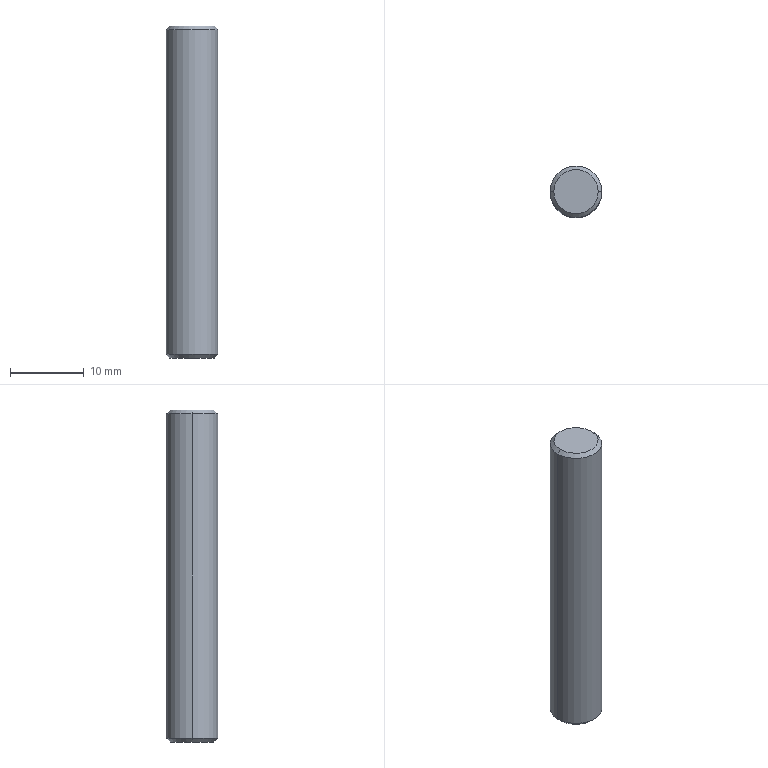Part | SolidWorks | features BaseBody 1 | 1 solid | 8 faces | box 7 x 7 x 45 mm | volume 1727 mm3 | cone 4 | cylinder 2 | plane 2 | commonest cylinder face diameters 7 x2
STEP:
#1=CARTESIAN_POINT('',(3.5,0.,0.5));
#2=VERTEX_POINT('',#1);
#3=CARTESIAN_POINT('',(-3.5,0.,0.5));
#4=VERTEX_POINT('',#3);
#5=CARTESIAN_POINT('',(0.,0.,0.5));
#6=DIRECTION('',(0.,0.,1.));
#7=DIRECTION('',(1.,0.,0.));
#8=AXIS2_PLACEMENT_3D('',#5,#6,#7);
#9=CIRCLE('',#8,3.5);
#10=EDGE_CURVE('',#2,#4,#9,.T.);
#11=ORIENTED_EDGE('',*,*,#10,.T.);
#12=CARTESIAN_POINT('',(-3.5,0.,44.5));
#13=VERTEX_POINT('',#12);
#14=CARTESIAN_POINT('',(-3.5,0.,0.));
#15=DIRECTION('',(0.,0.,1.));
#16=VECTOR('',#15,1000.);
#17=LINE('',#14,#16);
#18=EDGE_CURVE('',#4,#13,#17,.T.);
#19=ORIENTED_EDGE('',*,*,#18,.T.);
#20=CARTESIAN_POINT('',(3.5,0.,44.5));
#21=VERTEX_POINT('',#20);
#22=CARTESIAN_POINT('',(0.,0.,44.5));
#23=DIRECTION('',(0.,0.,-1.));
#24=DIRECTION('',(1.,0.,0.));
#25=AXIS2_PLACEMENT_3D('',#22,#23,#24);
#26=CIRCLE('',#25,3.5);
#27=EDGE_CURVE('',#13,#21,#26,.T.);
#28=ORIENTED_EDGE('',*,*,#27,.T.);
#29=CARTESIAN_POINT('',(3.5,0.,0.));
#30=DIRECTION('',(0.,0.,1.));
#31=VECTOR('',#30,1000.);
#32=LINE('',#29,#31);
#33=EDGE_CURVE('',#2,#21,#32,.T.);
#34=ORIENTED_EDGE('',*,*,#33,.F.);
#35=EDGE_LOOP('',(#11,#19,#28,#34));
#36=FACE_OUTER_BOUND('',#35,.T.);
#37=CARTESIAN_POINT('',(0.,0.,0.));
#38=DIRECTION('',(0.,0.,1.));
#39=DIRECTION('',(1.,0.,0.));
#40=AXIS2_PLACEMENT_3D('',#37,#38,#39);
#41=CYLINDRICAL_SURFACE('',#40,3.5);
#42=ADVANCED_FACE('',(#36),#41,.T.);
#43=CARTESIAN_POINT('',(-3.,0.,45.));
#44=VERTEX_POINT('',#43);
#45=CARTESIAN_POINT('',(3.,0.,45.));
#46=VERTEX_POINT('',#45);
#47=CARTESIAN_POINT('',(0.,0.,45.));
#48=DIRECTION('',(0.,0.,-1.));
#49=DIRECTION('',(-1.,0.,0.));
#50=AXIS2_PLACEMENT_3D('',#47,#48,#49);
#51=CIRCLE('',#50,3.);
#52=EDGE_CURVE('',#44,#46,#51,.T.);
#53=ORIENTED_EDGE('',*,*,#52,.T.);
#54=CARTESIAN_POINT('',(3.5,0.,44.5));
#55=DIRECTION('',(0.7071,0.,-0.7071));
#56=VECTOR('',#55,1000.);
#57=LINE('',#54,#56);
#58=EDGE_CURVE('',#46,#21,#57,.T.);
#59=ORIENTED_EDGE('',*,*,#58,.T.);
#60=ORIENTED_EDGE('',*,*,#27,.F.);
#61=CARTESIAN_POINT('',(-3.5,0.,44.5));
#62=DIRECTION('',(-0.7071,0.,-0.7071));
#63=VECTOR('',#62,1000.);
#64=LINE('',#61,#63);
#65=EDGE_CURVE('',#44,#13,#64,.T.);
#66=ORIENTED_EDGE('',*,*,#65,.F.);
#67=EDGE_LOOP('',(#53,#59,#60,#66));
#68=FACE_OUTER_BOUND('',#67,.T.);
#69=CARTESIAN_POINT('',(0.,0.,44.5));
#70=DIRECTION('',(0.,0.,-1.));
#71=DIRECTION('',(-1.,0.,0.));
#72=AXIS2_PLACEMENT_3D('',#69,#70,#71);
#73=CONICAL_SURFACE('',#72,3.5,0.7854);
#74=ADVANCED_FACE('',(#68),#73,.T.);
#75=CARTESIAN_POINT('',(3.,0.,0.));
#76=VERTEX_POINT('',#75);
#77=CARTESIAN_POINT('',(-3.,0.,0.));
#78=VERTEX_POINT('',#77);
#79=CARTESIAN_POINT('',(0.,0.,0.));
#80=DIRECTION('',(0.,0.,1.));
#81=DIRECTION('',(1.,0.,0.));
#82=AXIS2_PLACEMENT_3D('',#79,#80,#81);
#83=CIRCLE('',#82,3.);
#84=EDGE_CURVE('',#76,#78,#83,.T.);
#85=ORIENTED_EDGE('',*,*,#84,.T.);
#86=CARTESIAN_POINT('',(-3.5,0.,0.5));
#87=DIRECTION('',(-0.7071,0.,0.7071));
#88=VECTOR('',#87,1000.);
#89=LINE('',#86,#88);
#90=EDGE_CURVE('',#78,#4,#89,.T.);
#91=ORIENTED_EDGE('',*,*,#90,.T.);
#92=ORIENTED_EDGE('',*,*,#10,.F.);
#93=CARTESIAN_POINT('',(3.5,0.,0.5));
#94=DIRECTION('',(0.7071,0.,0.7071));
#95=VECTOR('',#94,1000.);
#96=LINE('',#93,#95);
#97=EDGE_CURVE('',#76,#2,#96,.T.);
#98=ORIENTED_EDGE('',*,*,#97,.F.);
#99=EDGE_LOOP('',(#85,#91,#92,#98));
#100=FACE_OUTER_BOUND('',#99,.T.);
#101=CARTESIAN_POINT('',(0.,0.,0.5));
#102=DIRECTION('',(0.,0.,1.));
#103=DIRECTION('',(1.,0.,0.));
#104=AXIS2_PLACEMENT_3D('',#101,#102,#103);
#105=CONICAL_SURFACE('',#104,3.5,0.7854);
#106=ADVANCED_FACE('',(#100),#105,.T.);
#107=ORIENTED_EDGE('',*,*,#18,.F.);
#108=CARTESIAN_POINT('',(0.,0.,0.5));
#109=DIRECTION('',(0.,0.,1.));
#110=DIRECTION('',(1.,0.,0.));
#111=AXIS2_PLACEMENT_3D('',#108,#109,#110);
#112=CIRCLE('',#111,3.5);
#113=EDGE_CURVE('',#4,#2,#112,.T.);
#114=ORIENTED_EDGE('',*,*,#113,.T.);
#115=ORIENTED_EDGE('',*,*,#33,.T.);
#116=CARTESIAN_POINT('',(0.,0.,44.5));
#117=DIRECTION('',(0.,0.,-1.));
#118=DIRECTION('',(1.,0.,0.));
#119=AXIS2_PLACEMENT_3D('',#116,#117,#118);
#120=CIRCLE('',#119,3.5);
#121=EDGE_CURVE('',#21,#13,#120,.T.);
#122=ORIENTED_EDGE('',*,*,#121,.T.);
#123=EDGE_LOOP('',(#107,#114,#115,#122));
#124=FACE_OUTER_BOUND('',#123,.T.);
#125=CARTESIAN_POINT('',(0.,0.,0.));
#126=DIRECTION('',(0.,0.,1.));
#127=DIRECTION('',(1.,0.,0.));
#128=AXIS2_PLACEMENT_3D('',#125,#126,#127);
#129=CYLINDRICAL_SURFACE('',#128,3.5);
#130=ADVANCED_FACE('',(#124),#129,.T.);
#131=ORIENTED_EDGE('',*,*,#58,.F.);
#132=CARTESIAN_POINT('',(0.,0.,45.));
#133=DIRECTION('',(0.,0.,-1.));
#134=DIRECTION('',(-1.,0.,0.));
#135=AXIS2_PLACEMENT_3D('',#132,#133,#134);
#136=CIRCLE('',#135,3.);
#137=EDGE_CURVE('',#46,#44,#136,.T.);
#138=ORIENTED_EDGE('',*,*,#137,.T.);
#139=ORIENTED_EDGE('',*,*,#65,.T.);
#140=ORIENTED_EDGE('',*,*,#121,.F.);
#141=EDGE_LOOP('',(#131,#138,#139,#140));
#142=FACE_OUTER_BOUND('',#141,.T.);
#143=CARTESIAN_POINT('',(0.,0.,44.5));
#144=DIRECTION('',(0.,0.,-1.));
#145=DIRECTION('',(-1.,0.,0.));
#146=AXIS2_PLACEMENT_3D('',#143,#144,#145);
#147=CONICAL_SURFACE('',#146,3.5,0.7854);
#148=ADVANCED_FACE('',(#142),#147,.T.);
#149=ORIENTED_EDGE('',*,*,#90,.F.);
#150=CARTESIAN_POINT('',(0.,0.,0.));
#151=DIRECTION('',(0.,0.,1.));
#152=DIRECTION('',(1.,0.,0.));
#153=AXIS2_PLACEMENT_3D('',#150,#151,#152);
#154=CIRCLE('',#153,3.);
#155=EDGE_CURVE('',#78,#76,#154,.T.);
#156=ORIENTED_EDGE('',*,*,#155,.T.);
#157=ORIENTED_EDGE('',*,*,#97,.T.);
#158=ORIENTED_EDGE('',*,*,#113,.F.);
#159=EDGE_LOOP('',(#149,#156,#157,#158));
#160=FACE_OUTER_BOUND('',#159,.T.);
#161=CARTESIAN_POINT('',(0.,0.,0.5));
#162=DIRECTION('',(0.,0.,1.));
#163=DIRECTION('',(1.,0.,0.));
#164=AXIS2_PLACEMENT_3D('',#161,#162,#163);
#165=CONICAL_SURFACE('',#164,3.5,0.7854);
#166=ADVANCED_FACE('',(#160),#165,.T.);
#167=ORIENTED_EDGE('',*,*,#52,.F.);
#168=ORIENTED_EDGE('',*,*,#137,.F.);
#169=EDGE_LOOP('',(#167,#168));
#170=FACE_OUTER_BOUND('',#169,.T.);
#171=CARTESIAN_POINT('',(0.,0.,45.));
#172=DIRECTION('',(0.,0.,1.));
#173=DIRECTION('',(1.,0.,0.));
#174=AXIS2_PLACEMENT_3D('',#171,#172,#173);
#175=PLANE('',#174);
#176=ADVANCED_FACE('',(#170),#175,.T.);
#177=ORIENTED_EDGE('',*,*,#84,.F.);
#178=ORIENTED_EDGE('',*,*,#155,.F.);
#179=EDGE_LOOP('',(#177,#178));
#180=FACE_OUTER_BOUND('',#179,.T.);
#181=CARTESIAN_POINT('',(0.,0.,0.));
#182=DIRECTION('',(0.,0.,1.));
#183=DIRECTION('',(1.,0.,0.));
#184=AXIS2_PLACEMENT_3D('',#181,#182,#183);
#185=PLANE('',#184);
#186=ADVANCED_FACE('',(#180),#185,.F.);
#187=CLOSED_SHELL('',(#42,#74,#106,#130,#148,#166,#176,#186));
#188=MANIFOLD_SOLID_BREP('',#187);
#189=CARTESIAN_POINT('',(0.,0.,0.));
#190=DIRECTION('',(0.,0.,1.));
#191=DIRECTION('',(1.,0.,0.));
#192=AXIS2_PLACEMENT_3D('',#189,#190,#191);
#193=(LENGTH_UNIT()NAMED_UNIT(*)SI_UNIT(.MILLI.,.METRE.));
#194=UNCERTAINTY_MEASURE_WITH_UNIT(LENGTH_MEASURE(0.00001),#193,'','');
#195=(NAMED_UNIT(*)PLANE_ANGLE_UNIT()SI_UNIT($,.RADIAN.));
#196=(NAMED_UNIT(*)SI_UNIT($,.STERADIAN.)SOLID_ANGLE_UNIT());
#197=(GEOMETRIC_REPRESENTATION_CONTEXT(3)GLOBAL_UNCERTAINTY_ASSIGNED_CONTEXT((#194))GLOBAL_UNIT_ASSIGNED_CONTEXT((#193,#195,#196))REPRESENTATION_CONTEXT('',''));
#198=ADVANCED_BREP_SHAPE_REPRESENTATION('',(#188,#192),#197);